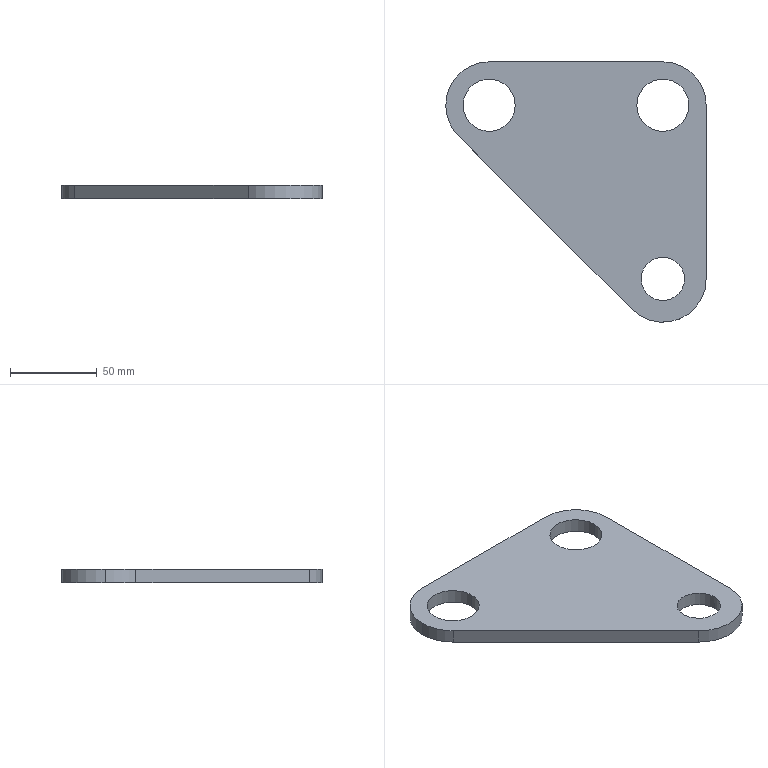Part | STEP file | 1 solid | 15 faces | box 150 x 150 x 8 mm | volume 108756 mm3 | cylinder 10 | plane 5 | commonest cylinder face diameters 30 x4 50 x4 25 x2
STEP:
#1=CARTESIAN_POINT('',(0.,0.,0.));
#2=DIRECTION('',(0.,0.,1.));
#3=DIRECTION('',(1.,0.,0.));
#4=AXIS2_PLACEMENT_3D('',#1,#2,#3);
#5=CARTESIAN_POINT('',(12.5,-100.,-4.));
#6=VERTEX_POINT('',#5);
#7=CARTESIAN_POINT('',(-12.5,-100.,-4.));
#8=VERTEX_POINT('',#7);
#9=CARTESIAN_POINT('',(0.,-100.,-4.));
#10=DIRECTION('',(0.,0.,1.));
#11=DIRECTION('',(1.,0.,0.));
#12=AXIS2_PLACEMENT_3D('',#9,#10,#11);
#13=CIRCLE('',#12,12.5);
#14=CARTESIAN_POINT('',(0.,-100.,4.));
#15=DIRECTION('',(0.,0.,-1.));
#16=DIRECTION('',(-1.,0.,0.));
#17=AXIS2_PLACEMENT_3D('',#14,#15,#16);
#18=CYLINDRICAL_SURFACE('',#17,12.5);
#19=CARTESIAN_POINT('',(3.142,8.));
#20=DIRECTION('',(-1.,0.));
#21=VECTOR('',#20,1.);
#22=LINE('',#19,#21);
#23=(GEOMETRIC_REPRESENTATION_CONTEXT(2)PARAMETRIC_REPRESENTATION_CONTEXT()REPRESENTATION_CONTEXT('',''));
#24=DEFINITIONAL_REPRESENTATION('',(#22),#23);
#25=PCURVE('',#18,#24);
#26=CARTESIAN_POINT('',(0.,-100.,-4.));
#27=DIRECTION('',(0.,0.,1.));
#28=DIRECTION('',(1.,0.,0.));
#29=AXIS2_PLACEMENT_3D('',#26,#27,#28);
#30=PLANE('',#29);
#31=CARTESIAN_POINT('',(0.,0.));
#32=DIRECTION('',(1.,0.));
#33=AXIS2_PLACEMENT_2D('',#31,#32);
#34=CIRCLE('',#33,12.5);
#35=(GEOMETRIC_REPRESENTATION_CONTEXT(2)PARAMETRIC_REPRESENTATION_CONTEXT()REPRESENTATION_CONTEXT('',''));
#36=DEFINITIONAL_REPRESENTATION('',(#34),#35);
#37=PCURVE('',#30,#36);
#38=SURFACE_CURVE('',#13,(#25,#37),.PCURVE_S1.);
#39=EDGE_CURVE('',#6,#8,#38,.T.);
#40=ORIENTED_EDGE('',*,*,#39,.T.);
#41=CARTESIAN_POINT('',(-12.5,-100.,4.));
#42=VERTEX_POINT('',#41);
#43=CARTESIAN_POINT('',(-12.5,-100.,4.));
#44=DIRECTION('',(0.,0.,-1.));
#45=VECTOR('',#44,1.);
#46=LINE('',#43,#45);
#47=CARTESIAN_POINT('',(0.,0.));
#48=DIRECTION('',(0.,1.));
#49=VECTOR('',#48,1.);
#50=LINE('',#47,#49);
#51=(GEOMETRIC_REPRESENTATION_CONTEXT(2)PARAMETRIC_REPRESENTATION_CONTEXT()REPRESENTATION_CONTEXT('',''));
#52=DEFINITIONAL_REPRESENTATION('',(#50),#51);
#53=PCURVE('',#18,#52);
#54=CARTESIAN_POINT('',(0.,-100.,4.));
#55=DIRECTION('',(0.,0.,-1.));
#56=DIRECTION('',(-1.,0.,0.));
#57=AXIS2_PLACEMENT_3D('',#54,#55,#56);
#58=CYLINDRICAL_SURFACE('',#57,12.5);
#59=CARTESIAN_POINT('',(6.283,0.));
#60=DIRECTION('',(0.,1.));
#61=VECTOR('',#60,1.);
#62=LINE('',#59,#61);
#63=(GEOMETRIC_REPRESENTATION_CONTEXT(2)PARAMETRIC_REPRESENTATION_CONTEXT()REPRESENTATION_CONTEXT('',''));
#64=DEFINITIONAL_REPRESENTATION('',(#62),#63);
#65=PCURVE('',#58,#64);
#66=SURFACE_CURVE('',#46,(#53,#65),.PCURVE_S1.);
#67=EDGE_CURVE('',#42,#8,#66,.T.);
#68=ORIENTED_EDGE('',*,*,#67,.F.);
#69=CARTESIAN_POINT('',(12.5,-100.,4.));
#70=VERTEX_POINT('',#69);
#71=CARTESIAN_POINT('',(0.,-100.,4.));
#72=DIRECTION('',(0.,0.,1.));
#73=DIRECTION('',(1.,0.,0.));
#74=AXIS2_PLACEMENT_3D('',#71,#72,#73);
#75=CIRCLE('',#74,12.5);
#76=CARTESIAN_POINT('',(3.142,0.));
#77=DIRECTION('',(-1.,0.));
#78=VECTOR('',#77,1.);
#79=LINE('',#76,#78);
#80=(GEOMETRIC_REPRESENTATION_CONTEXT(2)PARAMETRIC_REPRESENTATION_CONTEXT()REPRESENTATION_CONTEXT('',''));
#81=DEFINITIONAL_REPRESENTATION('',(#79),#80);
#82=PCURVE('',#18,#81);
#83=CARTESIAN_POINT('',(0.,-100.,4.));
#84=DIRECTION('',(0.,0.,1.));
#85=DIRECTION('',(1.,0.,0.));
#86=AXIS2_PLACEMENT_3D('',#83,#84,#85);
#87=PLANE('',#86);
#88=CARTESIAN_POINT('',(0.,0.));
#89=DIRECTION('',(1.,0.));
#90=AXIS2_PLACEMENT_2D('',#88,#89);
#91=CIRCLE('',#90,12.5);
#92=(GEOMETRIC_REPRESENTATION_CONTEXT(2)PARAMETRIC_REPRESENTATION_CONTEXT()REPRESENTATION_CONTEXT('',''));
#93=DEFINITIONAL_REPRESENTATION('',(#91),#92);
#94=PCURVE('',#87,#93);
#95=SURFACE_CURVE('',#75,(#82,#94),.PCURVE_S1.);
#96=EDGE_CURVE('',#70,#42,#95,.T.);
#97=ORIENTED_EDGE('',*,*,#96,.F.);
#98=CARTESIAN_POINT('',(12.5,-100.,4.));
#99=DIRECTION('',(0.,0.,-1.));
#100=VECTOR('',#99,1.);
#101=LINE('',#98,#100);
#102=CARTESIAN_POINT('',(3.142,0.));
#103=DIRECTION('',(0.,1.));
#104=VECTOR('',#103,1.);
#105=LINE('',#102,#104);
#106=(GEOMETRIC_REPRESENTATION_CONTEXT(2)PARAMETRIC_REPRESENTATION_CONTEXT()REPRESENTATION_CONTEXT('',''));
#107=DEFINITIONAL_REPRESENTATION('',(#105),#106);
#108=PCURVE('',#18,#107);
#109=CARTESIAN_POINT('',(3.142,0.));
#110=DIRECTION('',(0.,1.));
#111=VECTOR('',#110,1.);
#112=LINE('',#109,#111);
#113=(GEOMETRIC_REPRESENTATION_CONTEXT(2)PARAMETRIC_REPRESENTATION_CONTEXT()REPRESENTATION_CONTEXT('',''));
#114=DEFINITIONAL_REPRESENTATION('',(#112),#113);
#115=PCURVE('',#58,#114);
#116=SURFACE_CURVE('',#101,(#108,#115),.PCURVE_S1.);
#117=EDGE_CURVE('',#70,#6,#116,.T.);
#118=ORIENTED_EDGE('',*,*,#117,.T.);
#119=EDGE_LOOP('',(#40,#68,#97,#118));
#120=FACE_BOUND('',#119,.F.);
#121=ADVANCED_FACE('',(#120),#18,.F.);
#122=CARTESIAN_POINT('',(-85.,0.,-4.));
#123=VERTEX_POINT('',#122);
#124=CARTESIAN_POINT('',(-115.,0.,-4.));
#125=VERTEX_POINT('',#124);
#126=CARTESIAN_POINT('',(-100.,0.,-4.));
#127=DIRECTION('',(0.,0.,1.));
#128=DIRECTION('',(1.,0.,0.));
#129=AXIS2_PLACEMENT_3D('',#126,#127,#128);
#130=CIRCLE('',#129,15.);
#131=CARTESIAN_POINT('',(-100.,0.,4.));
#132=DIRECTION('',(0.,0.,-1.));
#133=DIRECTION('',(-1.,0.,0.));
#134=AXIS2_PLACEMENT_3D('',#131,#132,#133);
#135=CYLINDRICAL_SURFACE('',#134,15.);
#136=CARTESIAN_POINT('',(3.142,8.));
#137=DIRECTION('',(-1.,0.));
#138=VECTOR('',#137,1.);
#139=LINE('',#136,#138);
#140=(GEOMETRIC_REPRESENTATION_CONTEXT(2)PARAMETRIC_REPRESENTATION_CONTEXT()REPRESENTATION_CONTEXT('',''));
#141=DEFINITIONAL_REPRESENTATION('',(#139),#140);
#142=PCURVE('',#135,#141);
#143=CARTESIAN_POINT('',(-100.,100.));
#144=DIRECTION('',(1.,0.));
#145=AXIS2_PLACEMENT_2D('',#143,#144);
#146=CIRCLE('',#145,15.);
#147=(GEOMETRIC_REPRESENTATION_CONTEXT(2)PARAMETRIC_REPRESENTATION_CONTEXT()REPRESENTATION_CONTEXT('',''));
#148=DEFINITIONAL_REPRESENTATION('',(#146),#147);
#149=PCURVE('',#30,#148);
#150=SURFACE_CURVE('',#130,(#142,#149),.PCURVE_S1.);
#151=EDGE_CURVE('',#123,#125,#150,.T.);
#152=ORIENTED_EDGE('',*,*,#151,.T.);
#153=CARTESIAN_POINT('',(-115.,0.,4.));
#154=VERTEX_POINT('',#153);
#155=CARTESIAN_POINT('',(-115.,0.,4.));
#156=DIRECTION('',(0.,0.,-1.));
#157=VECTOR('',#156,1.);
#158=LINE('',#155,#157);
#159=CARTESIAN_POINT('',(0.,0.));
#160=DIRECTION('',(0.,1.));
#161=VECTOR('',#160,1.);
#162=LINE('',#159,#161);
#163=(GEOMETRIC_REPRESENTATION_CONTEXT(2)PARAMETRIC_REPRESENTATION_CONTEXT()REPRESENTATION_CONTEXT('',''));
#164=DEFINITIONAL_REPRESENTATION('',(#162),#163);
#165=PCURVE('',#135,#164);
#166=CARTESIAN_POINT('',(-100.,0.,4.));
#167=DIRECTION('',(0.,0.,-1.));
#168=DIRECTION('',(-1.,0.,0.));
#169=AXIS2_PLACEMENT_3D('',#166,#167,#168);
#170=CYLINDRICAL_SURFACE('',#169,15.);
#171=CARTESIAN_POINT('',(6.283,0.));
#172=DIRECTION('',(0.,1.));
#173=VECTOR('',#172,1.);
#174=LINE('',#171,#173);
#175=(GEOMETRIC_REPRESENTATION_CONTEXT(2)PARAMETRIC_REPRESENTATION_CONTEXT()REPRESENTATION_CONTEXT('',''));
#176=DEFINITIONAL_REPRESENTATION('',(#174),#175);
#177=PCURVE('',#170,#176);
#178=SURFACE_CURVE('',#158,(#165,#177),.PCURVE_S1.);
#179=EDGE_CURVE('',#154,#125,#178,.T.);
#180=ORIENTED_EDGE('',*,*,#179,.F.);
#181=CARTESIAN_POINT('',(-85.,0.,4.));
#182=VERTEX_POINT('',#181);
#183=CARTESIAN_POINT('',(-100.,0.,4.));
#184=DIRECTION('',(0.,0.,1.));
#185=DIRECTION('',(1.,0.,0.));
#186=AXIS2_PLACEMENT_3D('',#183,#184,#185);
#187=CIRCLE('',#186,15.);
#188=CARTESIAN_POINT('',(3.142,0.));
#189=DIRECTION('',(-1.,0.));
#190=VECTOR('',#189,1.);
#191=LINE('',#188,#190);
#192=(GEOMETRIC_REPRESENTATION_CONTEXT(2)PARAMETRIC_REPRESENTATION_CONTEXT()REPRESENTATION_CONTEXT('',''));
#193=DEFINITIONAL_REPRESENTATION('',(#191),#192);
#194=PCURVE('',#135,#193);
#195=CARTESIAN_POINT('',(-100.,100.));
#196=DIRECTION('',(1.,0.));
#197=AXIS2_PLACEMENT_2D('',#195,#196);
#198=CIRCLE('',#197,15.);
#199=(GEOMETRIC_REPRESENTATION_CONTEXT(2)PARAMETRIC_REPRESENTATION_CONTEXT()REPRESENTATION_CONTEXT('',''));
#200=DEFINITIONAL_REPRESENTATION('',(#198),#199);
#201=PCURVE('',#87,#200);
#202=SURFACE_CURVE('',#187,(#194,#201),.PCURVE_S1.);
#203=EDGE_CURVE('',#182,#154,#202,.T.);
#204=ORIENTED_EDGE('',*,*,#203,.F.);
#205=CARTESIAN_POINT('',(-85.,0.,4.));
#206=DIRECTION('',(0.,0.,-1.));
#207=VECTOR('',#206,1.);
#208=LINE('',#205,#207);
#209=CARTESIAN_POINT('',(3.142,0.));
#210=DIRECTION('',(0.,1.));
#211=VECTOR('',#210,1.);
#212=LINE('',#209,#211);
#213=(GEOMETRIC_REPRESENTATION_CONTEXT(2)PARAMETRIC_REPRESENTATION_CONTEXT()REPRESENTATION_CONTEXT('',''));
#214=DEFINITIONAL_REPRESENTATION('',(#212),#213);
#215=PCURVE('',#135,#214);
#216=CARTESIAN_POINT('',(3.142,0.));
#217=DIRECTION('',(0.,1.));
#218=VECTOR('',#217,1.);
#219=LINE('',#216,#218);
#220=(GEOMETRIC_REPRESENTATION_CONTEXT(2)PARAMETRIC_REPRESENTATION_CONTEXT()REPRESENTATION_CONTEXT('',''));
#221=DEFINITIONAL_REPRESENTATION('',(#219),#220);
#222=PCURVE('',#170,#221);
#223=SURFACE_CURVE('',#208,(#215,#222),.PCURVE_S1.);
#224=EDGE_CURVE('',#182,#123,#223,.T.);
#225=ORIENTED_EDGE('',*,*,#224,.T.);
#226=EDGE_LOOP('',(#152,#180,#204,#225));
#227=FACE_BOUND('',#226,.F.);
#228=ADVANCED_FACE('',(#227),#135,.F.);
#229=CARTESIAN_POINT('',(15.,0.,-4.));
#230=VERTEX_POINT('',#229);
#231=CARTESIAN_POINT('',(-15.,0.,-4.));
#232=VERTEX_POINT('',#231);
#233=CARTESIAN_POINT('',(0.,0.,-4.));
#234=DIRECTION('',(0.,0.,1.));
#235=DIRECTION('',(1.,0.,0.));
#236=AXIS2_PLACEMENT_3D('',#233,#234,#235);
#237=CIRCLE('',#236,15.);
#238=CARTESIAN_POINT('',(0.,0.,4.));
#239=DIRECTION('',(0.,0.,-1.));
#240=DIRECTION('',(-1.,0.,0.));
#241=AXIS2_PLACEMENT_3D('',#238,#239,#240);
#242=CYLINDRICAL_SURFACE('',#241,15.);
#243=CARTESIAN_POINT('',(3.142,8.));
#244=DIRECTION('',(-1.,0.));
#245=VECTOR('',#244,1.);
#246=LINE('',#243,#245);
#247=(GEOMETRIC_REPRESENTATION_CONTEXT(2)PARAMETRIC_REPRESENTATION_CONTEXT()REPRESENTATION_CONTEXT('',''));
#248=DEFINITIONAL_REPRESENTATION('',(#246),#247);
#249=PCURVE('',#242,#248);
#250=CARTESIAN_POINT('',(0.,100.));
#251=DIRECTION('',(1.,0.));
#252=AXIS2_PLACEMENT_2D('',#250,#251);
#253=CIRCLE('',#252,15.);
#254=(GEOMETRIC_REPRESENTATION_CONTEXT(2)PARAMETRIC_REPRESENTATION_CONTEXT()REPRESENTATION_CONTEXT('',''));
#255=DEFINITIONAL_REPRESENTATION('',(#253),#254);
#256=PCURVE('',#30,#255);
#257=SURFACE_CURVE('',#237,(#249,#256),.PCURVE_S1.);
#258=EDGE_CURVE('',#230,#232,#257,.T.);
#259=ORIENTED_EDGE('',*,*,#258,.T.);
#260=CARTESIAN_POINT('',(-15.,0.,4.));
#261=VERTEX_POINT('',#260);
#262=CARTESIAN_POINT('',(-15.,0.,4.));
#263=DIRECTION('',(0.,0.,-1.));
#264=VECTOR('',#263,1.);
#265=LINE('',#262,#264);
#266=CARTESIAN_POINT('',(0.,0.));
#267=DIRECTION('',(0.,1.));
#268=VECTOR('',#267,1.);
#269=LINE('',#266,#268);
#270=(GEOMETRIC_REPRESENTATION_CONTEXT(2)PARAMETRIC_REPRESENTATION_CONTEXT()REPRESENTATION_CONTEXT('',''));
#271=DEFINITIONAL_REPRESENTATION('',(#269),#270);
#272=PCURVE('',#242,#271);
#273=CARTESIAN_POINT('',(0.,0.,4.));
#274=DIRECTION('',(0.,0.,-1.));
#275=DIRECTION('',(-1.,0.,0.));
#276=AXIS2_PLACEMENT_3D('',#273,#274,#275);
#277=CYLINDRICAL_SURFACE('',#276,15.);
#278=CARTESIAN_POINT('',(6.283,0.));
#279=DIRECTION('',(0.,1.));
#280=VECTOR('',#279,1.);
#281=LINE('',#278,#280);
#282=(GEOMETRIC_REPRESENTATION_CONTEXT(2)PARAMETRIC_REPRESENTATION_CONTEXT()REPRESENTATION_CONTEXT('',''));
#283=DEFINITIONAL_REPRESENTATION('',(#281),#282);
#284=PCURVE('',#277,#283);
#285=SURFACE_CURVE('',#265,(#272,#284),.PCURVE_S1.);
#286=EDGE_CURVE('',#261,#232,#285,.T.);
#287=ORIENTED_EDGE('',*,*,#286,.F.);
#288=CARTESIAN_POINT('',(15.,0.,4.));
#289=VERTEX_POINT('',#288);
#290=CARTESIAN_POINT('',(0.,0.,4.));
#291=DIRECTION('',(0.,0.,1.));
#292=DIRECTION('',(1.,0.,0.));
#293=AXIS2_PLACEMENT_3D('',#290,#291,#292);
#294=CIRCLE('',#293,15.);
#295=CARTESIAN_POINT('',(3.142,0.));
#296=DIRECTION('',(-1.,0.));
#297=VECTOR('',#296,1.);
#298=LINE('',#295,#297);
#299=(GEOMETRIC_REPRESENTATION_CONTEXT(2)PARAMETRIC_REPRESENTATION_CONTEXT()REPRESENTATION_CONTEXT('',''));
#300=DEFINITIONAL_REPRESENTATION('',(#298),#299);
#301=PCURVE('',#242,#300);
#302=CARTESIAN_POINT('',(0.,100.));
#303=DIRECTION('',(1.,0.));
#304=AXIS2_PLACEMENT_2D('',#302,#303);
#305=CIRCLE('',#304,15.);
#306=(GEOMETRIC_REPRESENTATION_CONTEXT(2)PARAMETRIC_REPRESENTATION_CONTEXT()REPRESENTATION_CONTEXT('',''));
#307=DEFINITIONAL_REPRESENTATION('',(#305),#306);
#308=PCURVE('',#87,#307);
#309=SURFACE_CURVE('',#294,(#301,#308),.PCURVE_S1.);
#310=EDGE_CURVE('',#289,#261,#309,.T.);
#311=ORIENTED_EDGE('',*,*,#310,.F.);
#312=CARTESIAN_POINT('',(15.,0.,4.));
#313=DIRECTION('',(0.,0.,-1.));
#314=VECTOR('',#313,1.);
#315=LINE('',#312,#314);
#316=CARTESIAN_POINT('',(3.142,0.));
#317=DIRECTION('',(0.,1.));
#318=VECTOR('',#317,1.);
#319=LINE('',#316,#318);
#320=(GEOMETRIC_REPRESENTATION_CONTEXT(2)PARAMETRIC_REPRESENTATION_CONTEXT()REPRESENTATION_CONTEXT('',''));
#321=DEFINITIONAL_REPRESENTATION('',(#319),#320);
#322=PCURVE('',#242,#321);
#323=CARTESIAN_POINT('',(3.142,0.));
#324=DIRECTION('',(0.,1.));
#325=VECTOR('',#324,1.);
#326=LINE('',#323,#325);
#327=(GEOMETRIC_REPRESENTATION_CONTEXT(2)PARAMETRIC_REPRESENTATION_CONTEXT()REPRESENTATION_CONTEXT('',''));
#328=DEFINITIONAL_REPRESENTATION('',(#326),#327);
#329=PCURVE('',#277,#328);
#330=SURFACE_CURVE('',#315,(#322,#329),.PCURVE_S1.);
#331=EDGE_CURVE('',#289,#230,#330,.T.);
#332=ORIENTED_EDGE('',*,*,#331,.T.);
#333=EDGE_LOOP('',(#259,#287,#311,#332));
#334=FACE_BOUND('',#333,.F.);
#335=ADVANCED_FACE('',(#334),#242,.F.);
#336=CARTESIAN_POINT('',(-117.678,-17.678,-4.));
#337=VERTEX_POINT('',#336);
#338=CARTESIAN_POINT('',(-17.678,-117.678,-4.));
#339=VERTEX_POINT('',#338);
#340=CARTESIAN_POINT('',(-117.678,-17.678,-4.));
#341=DIRECTION('',(0.7071,-0.7071,0.));
#342=VECTOR('',#341,1.);
#343=LINE('',#340,#342);
#344=CARTESIAN_POINT('',(-117.678,-17.678,4.));
#345=DIRECTION('',(0.7071,0.7071,0.));
#346=DIRECTION('',(0.,0.,-1.));
#347=AXIS2_PLACEMENT_3D('',#344,#345,#346);
#348=PLANE('',#347);
#349=CARTESIAN_POINT('',(8.,0.));
#350=DIRECTION('',(0.,-1.));
#351=VECTOR('',#350,1.);
#352=LINE('',#349,#351);
#353=(GEOMETRIC_REPRESENTATION_CONTEXT(2)PARAMETRIC_REPRESENTATION_CONTEXT()REPRESENTATION_CONTEXT('',''));
#354=DEFINITIONAL_REPRESENTATION('',(#352),#353);
#355=PCURVE('',#348,#354);
#356=CARTESIAN_POINT('',(-117.678,82.322));
#357=DIRECTION('',(0.7071,-0.7071));
#358=VECTOR('',#357,1.);
#359=LINE('',#356,#358);
#360=(GEOMETRIC_REPRESENTATION_CONTEXT(2)PARAMETRIC_REPRESENTATION_CONTEXT()REPRESENTATION_CONTEXT('',''));
#361=DEFINITIONAL_REPRESENTATION('',(#359),#360);
#362=PCURVE('',#30,#361);
#363=SURFACE_CURVE('',#343,(#355,#362),.PCURVE_S1.);
#364=EDGE_CURVE('',#337,#339,#363,.T.);
#365=ORIENTED_EDGE('',*,*,#364,.T.);
#366=CARTESIAN_POINT('',(-17.678,-117.678,4.));
#367=VERTEX_POINT('',#366);
#368=CARTESIAN_POINT('',(-17.678,-117.678,4.));
#369=DIRECTION('',(0.,0.,-1.));
#370=VECTOR('',#369,1.);
#371=LINE('',#368,#370);
#372=CARTESIAN_POINT('',(0.,-141.421));
#373=DIRECTION('',(1.,0.));
#374=VECTOR('',#373,1.);
#375=LINE('',#372,#374);
#376=(GEOMETRIC_REPRESENTATION_CONTEXT(2)PARAMETRIC_REPRESENTATION_CONTEXT()REPRESENTATION_CONTEXT('',''));
#377=DEFINITIONAL_REPRESENTATION('',(#375),#376);
#378=PCURVE('',#348,#377);
#379=CARTESIAN_POINT('',(0.,-100.,4.));
#380=DIRECTION('',(0.,0.,-1.));
#381=DIRECTION('',(-1.,0.,0.));
#382=AXIS2_PLACEMENT_3D('',#379,#380,#381);
#383=CYLINDRICAL_SURFACE('',#382,25.);
#384=CARTESIAN_POINT('',(5.498,0.));
#385=DIRECTION('',(0.,1.));
#386=VECTOR('',#385,1.);
#387=LINE('',#384,#386);
#388=(GEOMETRIC_REPRESENTATION_CONTEXT(2)PARAMETRIC_REPRESENTATION_CONTEXT()REPRESENTATION_CONTEXT('',''));
#389=DEFINITIONAL_REPRESENTATION('',(#387),#388);
#390=PCURVE('',#383,#389);
#391=SURFACE_CURVE('',#371,(#378,#390),.PCURVE_S1.);
#392=EDGE_CURVE('',#367,#339,#391,.T.);
#393=ORIENTED_EDGE('',*,*,#392,.F.);
#394=CARTESIAN_POINT('',(-117.678,-17.678,4.));
#395=VERTEX_POINT('',#394);
#396=CARTESIAN_POINT('',(-117.678,-17.678,4.));
#397=DIRECTION('',(0.7071,-0.7071,0.));
#398=VECTOR('',#397,1.);
#399=LINE('',#396,#398);
#400=CARTESIAN_POINT('',(0.,0.));
#401=DIRECTION('',(0.,-1.));
#402=VECTOR('',#401,1.);
#403=LINE('',#400,#402);
#404=(GEOMETRIC_REPRESENTATION_CONTEXT(2)PARAMETRIC_REPRESENTATION_CONTEXT()REPRESENTATION_CONTEXT('',''));
#405=DEFINITIONAL_REPRESENTATION('',(#403),#404);
#406=PCURVE('',#348,#405);
#407=CARTESIAN_POINT('',(-117.678,82.322));
#408=DIRECTION('',(0.7071,-0.7071));
#409=VECTOR('',#408,1.);
#410=LINE('',#407,#409);
#411=(GEOMETRIC_REPRESENTATION_CONTEXT(2)PARAMETRIC_REPRESENTATION_CONTEXT()REPRESENTATION_CONTEXT('',''));
#412=DEFINITIONAL_REPRESENTATION('',(#410),#411);
#413=PCURVE('',#87,#412);
#414=SURFACE_CURVE('',#399,(#406,#413),.PCURVE_S1.);
#415=EDGE_CURVE('',#395,#367,#414,.T.);
#416=ORIENTED_EDGE('',*,*,#415,.F.);
#417=CARTESIAN_POINT('',(-117.678,-17.678,4.));
#418=DIRECTION('',(0.,0.,-1.));
#419=VECTOR('',#418,1.);
#420=LINE('',#417,#419);
#421=CARTESIAN_POINT('',(0.,0.));
#422=DIRECTION('',(1.,0.));
#423=VECTOR('',#422,1.);
#424=LINE('',#421,#423);
#425=(GEOMETRIC_REPRESENTATION_CONTEXT(2)PARAMETRIC_REPRESENTATION_CONTEXT()REPRESENTATION_CONTEXT('',''));
#426=DEFINITIONAL_REPRESENTATION('',(#424),#425);
#427=PCURVE('',#348,#426);
#428=CARTESIAN_POINT('',(-100.,0.,4.));
#429=DIRECTION('',(0.,0.,-1.));
#430=DIRECTION('',(-1.,0.,0.));
#431=AXIS2_PLACEMENT_3D('',#428,#429,#430);
#432=CYLINDRICAL_SURFACE('',#431,25.);
#433=CARTESIAN_POINT('',(5.498,0.));
#434=DIRECTION('',(0.,1.));
#435=VECTOR('',#434,1.);
#436=LINE('',#433,#435);
#437=(GEOMETRIC_REPRESENTATION_CONTEXT(2)PARAMETRIC_REPRESENTATION_CONTEXT()REPRESENTATION_CONTEXT('',''));
#438=DEFINITIONAL_REPRESENTATION('',(#436),#437);
#439=PCURVE('',#432,#438);
#440=SURFACE_CURVE('',#420,(#427,#439),.PCURVE_S1.);
#441=EDGE_CURVE('',#395,#337,#440,.T.);
#442=ORIENTED_EDGE('',*,*,#441,.T.);
#443=EDGE_LOOP('',(#365,#393,#416,#442));
#444=FACE_BOUND('',#443,.T.);
#445=ADVANCED_FACE('',(#444),#348,.F.);
#446=CARTESIAN_POINT('',(-125.,0.,4.));
#447=VERTEX_POINT('',#446);
#448=CARTESIAN_POINT('',(-125.,0.,-4.));
#449=VERTEX_POINT('',#448);
#450=CARTESIAN_POINT('',(-125.,0.,4.));
#451=DIRECTION('',(0.,0.,-1.));
#452=VECTOR('',#451,1.);
#453=LINE('',#450,#452);
#454=CARTESIAN_POINT('',(-100.,0.,4.));
#455=DIRECTION('',(0.,0.,-1.));
#456=DIRECTION('',(-1.,0.,0.));
#457=AXIS2_PLACEMENT_3D('',#454,#455,#456);
#458=CYLINDRICAL_SURFACE('',#457,25.);
#459=CARTESIAN_POINT('',(0.,0.));
#460=DIRECTION('',(0.,1.));
#461=VECTOR('',#460,1.);
#462=LINE('',#459,#461);
#463=(GEOMETRIC_REPRESENTATION_CONTEXT(2)PARAMETRIC_REPRESENTATION_CONTEXT()REPRESENTATION_CONTEXT('',''));
#464=DEFINITIONAL_REPRESENTATION('',(#462),#463);
#465=PCURVE('',#458,#464);
#466=CARTESIAN_POINT('',(6.283,0.));
#467=DIRECTION('',(0.,1.));
#468=VECTOR('',#467,1.);
#469=LINE('',#466,#468);
#470=(GEOMETRIC_REPRESENTATION_CONTEXT(2)PARAMETRIC_REPRESENTATION_CONTEXT()REPRESENTATION_CONTEXT('',''));
#471=DEFINITIONAL_REPRESENTATION('',(#469),#470);
#472=PCURVE('',#432,#471);
#473=SURFACE_CURVE('',#453,(#465,#472),.PCURVE_S1.);
#474=EDGE_CURVE('',#447,#449,#473,.T.);
#475=ORIENTED_EDGE('',*,*,#474,.F.);
#476=CARTESIAN_POINT('',(-100.,25.,4.));
#477=VERTEX_POINT('',#476);
#478=CARTESIAN_POINT('',(-100.,0.,4.));
#479=DIRECTION('',(0.,0.,1.));
#480=DIRECTION('',(1.,0.,0.));
#481=AXIS2_PLACEMENT_3D('',#478,#479,#480);
#482=CIRCLE('',#481,25.);
#483=CARTESIAN_POINT('',(3.142,0.));
#484=DIRECTION('',(-1.,0.));
#485=VECTOR('',#484,1.);
#486=LINE('',#483,#485);
#487=(GEOMETRIC_REPRESENTATION_CONTEXT(2)PARAMETRIC_REPRESENTATION_CONTEXT()REPRESENTATION_CONTEXT('',''));
#488=DEFINITIONAL_REPRESENTATION('',(#486),#487);
#489=PCURVE('',#458,#488);
#490=CARTESIAN_POINT('',(-100.,100.));
#491=DIRECTION('',(1.,0.));
#492=AXIS2_PLACEMENT_2D('',#490,#491);
#493=CIRCLE('',#492,25.);
#494=(GEOMETRIC_REPRESENTATION_CONTEXT(2)PARAMETRIC_REPRESENTATION_CONTEXT()REPRESENTATION_CONTEXT('',''));
#495=DEFINITIONAL_REPRESENTATION('',(#493),#494);
#496=PCURVE('',#87,#495);
#497=SURFACE_CURVE('',#482,(#489,#496),.PCURVE_S1.);
#498=EDGE_CURVE('',#477,#447,#497,.T.);
#499=ORIENTED_EDGE('',*,*,#498,.F.);
#500=CARTESIAN_POINT('',(-100.,25.,-4.));
#501=VERTEX_POINT('',#500);
#502=CARTESIAN_POINT('',(-100.,25.,4.));
#503=DIRECTION('',(0.,0.,-1.));
#504=VECTOR('',#503,1.);
#505=LINE('',#502,#504);
#506=CARTESIAN_POINT('',(1.571,0.));
#507=DIRECTION('',(0.,1.));
#508=VECTOR('',#507,1.);
#509=LINE('',#506,#508);
#510=(GEOMETRIC_REPRESENTATION_CONTEXT(2)PARAMETRIC_REPRESENTATION_CONTEXT()REPRESENTATION_CONTEXT('',''));
#511=DEFINITIONAL_REPRESENTATION('',(#509),#510);
#512=PCURVE('',#458,#511);
#513=CARTESIAN_POINT('',(-100.,25.,4.));
#514=DIRECTION('',(0.,-1.,0.));
#515=DIRECTION('',(0.,0.,-1.));
#516=AXIS2_PLACEMENT_3D('',#513,#514,#515);
#517=PLANE('',#516);
#518=CARTESIAN_POINT('',(0.,0.));
#519=DIRECTION('',(1.,0.));
#520=VECTOR('',#519,1.);
#521=LINE('',#518,#520);
#522=(GEOMETRIC_REPRESENTATION_CONTEXT(2)PARAMETRIC_REPRESENTATION_CONTEXT()REPRESENTATION_CONTEXT('',''));
#523=DEFINITIONAL_REPRESENTATION('',(#521),#522);
#524=PCURVE('',#517,#523);
#525=SURFACE_CURVE('',#505,(#512,#524),.PCURVE_S1.);
#526=EDGE_CURVE('',#477,#501,#525,.T.);
#527=ORIENTED_EDGE('',*,*,#526,.T.);
#528=CARTESIAN_POINT('',(-100.,0.,-4.));
#529=DIRECTION('',(0.,0.,1.));
#530=DIRECTION('',(1.,0.,0.));
#531=AXIS2_PLACEMENT_3D('',#528,#529,#530);
#532=CIRCLE('',#531,25.);
#533=CARTESIAN_POINT('',(3.142,8.));
#534=DIRECTION('',(-1.,0.));
#535=VECTOR('',#534,1.);
#536=LINE('',#533,#535);
#537=(GEOMETRIC_REPRESENTATION_CONTEXT(2)PARAMETRIC_REPRESENTATION_CONTEXT()REPRESENTATION_CONTEXT('',''));
#538=DEFINITIONAL_REPRESENTATION('',(#536),#537);
#539=PCURVE('',#458,#538);
#540=CARTESIAN_POINT('',(-100.,100.));
#541=DIRECTION('',(1.,0.));
#542=AXIS2_PLACEMENT_2D('',#540,#541);
#543=CIRCLE('',#542,25.);
#544=(GEOMETRIC_REPRESENTATION_CONTEXT(2)PARAMETRIC_REPRESENTATION_CONTEXT()REPRESENTATION_CONTEXT('',''));
#545=DEFINITIONAL_REPRESENTATION('',(#543),#544);
#546=PCURVE('',#30,#545);
#547=SURFACE_CURVE('',#532,(#539,#546),.PCURVE_S1.);
#548=EDGE_CURVE('',#501,#449,#547,.T.);
#549=ORIENTED_EDGE('',*,*,#548,.T.);
#550=EDGE_LOOP('',(#475,#499,#527,#549));
#551=FACE_BOUND('',#550,.T.);
#552=ADVANCED_FACE('',(#551),#458,.T.);
#553=CARTESIAN_POINT('',(0.,25.,-4.));
#554=VERTEX_POINT('',#553);
#555=CARTESIAN_POINT('',(-100.,25.,-4.));
#556=DIRECTION('',(-1.,0.,0.));
#557=VECTOR('',#556,1.);
#558=LINE('',#555,#557);
#559=CARTESIAN_POINT('',(8.,0.));
#560=DIRECTION('',(0.,-1.));
#561=VECTOR('',#560,1.);
#562=LINE('',#559,#561);
#563=(GEOMETRIC_REPRESENTATION_CONTEXT(2)PARAMETRIC_REPRESENTATION_CONTEXT()REPRESENTATION_CONTEXT('',''));
#564=DEFINITIONAL_REPRESENTATION('',(#562),#563);
#565=PCURVE('',#517,#564);
#566=CARTESIAN_POINT('',(-100.,125.));
#567=DIRECTION('',(-1.,0.));
#568=VECTOR('',#567,1.);
#569=LINE('',#566,#568);
#570=(GEOMETRIC_REPRESENTATION_CONTEXT(2)PARAMETRIC_REPRESENTATION_CONTEXT()REPRESENTATION_CONTEXT('',''));
#571=DEFINITIONAL_REPRESENTATION('',(#569),#570);
#572=PCURVE('',#30,#571);
#573=SURFACE_CURVE('',#558,(#565,#572),.PCURVE_S1.);
#574=EDGE_CURVE('',#554,#501,#573,.T.);
#575=ORIENTED_EDGE('',*,*,#574,.T.);
#576=ORIENTED_EDGE('',*,*,#526,.F.);
#577=CARTESIAN_POINT('',(0.,25.,4.));
#578=VERTEX_POINT('',#577);
#579=CARTESIAN_POINT('',(-100.,25.,4.));
#580=DIRECTION('',(-1.,0.,0.));
#581=VECTOR('',#580,1.);
#582=LINE('',#579,#581);
#583=CARTESIAN_POINT('',(0.,0.));
#584=DIRECTION('',(0.,-1.));
#585=VECTOR('',#584,1.);
#586=LINE('',#583,#585);
#587=(GEOMETRIC_REPRESENTATION_CONTEXT(2)PARAMETRIC_REPRESENTATION_CONTEXT()REPRESENTATION_CONTEXT('',''));
#588=DEFINITIONAL_REPRESENTATION('',(#586),#587);
#589=PCURVE('',#517,#588);
#590=CARTESIAN_POINT('',(-100.,125.));
#591=DIRECTION('',(-1.,0.));
#592=VECTOR('',#591,1.);
#593=LINE('',#590,#592);
#594=(GEOMETRIC_REPRESENTATION_CONTEXT(2)PARAMETRIC_REPRESENTATION_CONTEXT()REPRESENTATION_CONTEXT('',''));
#595=DEFINITIONAL_REPRESENTATION('',(#593),#594);
#596=PCURVE('',#87,#595);
#597=SURFACE_CURVE('',#582,(#589,#596),.PCURVE_S1.);
#598=EDGE_CURVE('',#578,#477,#597,.T.);
#599=ORIENTED_EDGE('',*,*,#598,.F.);
#600=CARTESIAN_POINT('',(0.,25.,4.));
#601=DIRECTION('',(0.,0.,-1.));
#602=VECTOR('',#601,1.);
#603=LINE('',#600,#602);
#604=CARTESIAN_POINT('',(0.,100.));
#605=DIRECTION('',(1.,0.));
#606=VECTOR('',#605,1.);
#607=LINE('',#604,#606);
#608=(GEOMETRIC_REPRESENTATION_CONTEXT(2)PARAMETRIC_REPRESENTATION_CONTEXT()REPRESENTATION_CONTEXT('',''));
#609=DEFINITIONAL_REPRESENTATION('',(#607),#608);
#610=PCURVE('',#517,#609);
#611=CARTESIAN_POINT('',(0.,0.,4.));
#612=DIRECTION('',(0.,0.,-1.));
#613=DIRECTION('',(-1.,0.,0.));
#614=AXIS2_PLACEMENT_3D('',#611,#612,#613);
#615=CYLINDRICAL_SURFACE('',#614,25.);
#616=CARTESIAN_POINT('',(1.571,0.));
#617=DIRECTION('',(0.,1.));
#618=VECTOR('',#617,1.);
#619=LINE('',#616,#618);
#620=(GEOMETRIC_REPRESENTATION_CONTEXT(2)PARAMETRIC_REPRESENTATION_CONTEXT()REPRESENTATION_CONTEXT('',''));
#621=DEFINITIONAL_REPRESENTATION('',(#619),#620);
#622=PCURVE('',#615,#621);
#623=SURFACE_CURVE('',#603,(#610,#622),.PCURVE_S1.);
#624=EDGE_CURVE('',#578,#554,#623,.T.);
#625=ORIENTED_EDGE('',*,*,#624,.T.);
#626=EDGE_LOOP('',(#575,#576,#599,#625));
#627=FACE_BOUND('',#626,.T.);
#628=ADVANCED_FACE('',(#627),#517,.F.);
#629=CARTESIAN_POINT('',(25.,0.,-4.));
#630=VERTEX_POINT('',#629);
#631=CARTESIAN_POINT('',(0.,0.,-4.));
#632=DIRECTION('',(0.,0.,1.));
#633=DIRECTION('',(1.,0.,0.));
#634=AXIS2_PLACEMENT_3D('',#631,#632,#633);
#635=CIRCLE('',#634,25.);
#636=CARTESIAN_POINT('',(3.142,8.));
#637=DIRECTION('',(-1.,0.));
#638=VECTOR('',#637,1.);
#639=LINE('',#636,#638);
#640=(GEOMETRIC_REPRESENTATION_CONTEXT(2)PARAMETRIC_REPRESENTATION_CONTEXT()REPRESENTATION_CONTEXT('',''));
#641=DEFINITIONAL_REPRESENTATION('',(#639),#640);
#642=PCURVE('',#615,#641);
#643=CARTESIAN_POINT('',(0.,100.));
#644=DIRECTION('',(1.,0.));
#645=AXIS2_PLACEMENT_2D('',#643,#644);
#646=CIRCLE('',#645,25.);
#647=(GEOMETRIC_REPRESENTATION_CONTEXT(2)PARAMETRIC_REPRESENTATION_CONTEXT()REPRESENTATION_CONTEXT('',''));
#648=DEFINITIONAL_REPRESENTATION('',(#646),#647);
#649=PCURVE('',#30,#648);
#650=SURFACE_CURVE('',#635,(#642,#649),.PCURVE_S1.);
#651=EDGE_CURVE('',#630,#554,#650,.T.);
#652=ORIENTED_EDGE('',*,*,#651,.T.);
#653=ORIENTED_EDGE('',*,*,#624,.F.);
#654=CARTESIAN_POINT('',(25.,0.,4.));
#655=VERTEX_POINT('',#654);
#656=CARTESIAN_POINT('',(0.,0.,4.));
#657=DIRECTION('',(0.,0.,1.));
#658=DIRECTION('',(1.,0.,0.));
#659=AXIS2_PLACEMENT_3D('',#656,#657,#658);
#660=CIRCLE('',#659,25.);
#661=CARTESIAN_POINT('',(3.142,0.));
#662=DIRECTION('',(-1.,0.));
#663=VECTOR('',#662,1.);
#664=LINE('',#661,#663);
#665=(GEOMETRIC_REPRESENTATION_CONTEXT(2)PARAMETRIC_REPRESENTATION_CONTEXT()REPRESENTATION_CONTEXT('',''));
#666=DEFINITIONAL_REPRESENTATION('',(#664),#665);
#667=PCURVE('',#615,#666);
#668=CARTESIAN_POINT('',(0.,100.));
#669=DIRECTION('',(1.,0.));
#670=AXIS2_PLACEMENT_2D('',#668,#669);
#671=CIRCLE('',#670,25.);
#672=(GEOMETRIC_REPRESENTATION_CONTEXT(2)PARAMETRIC_REPRESENTATION_CONTEXT()REPRESENTATION_CONTEXT('',''));
#673=DEFINITIONAL_REPRESENTATION('',(#671),#672);
#674=PCURVE('',#87,#673);
#675=SURFACE_CURVE('',#660,(#667,#674),.PCURVE_S1.);
#676=EDGE_CURVE('',#655,#578,#675,.T.);
#677=ORIENTED_EDGE('',*,*,#676,.F.);
#678=CARTESIAN_POINT('',(25.,0.,4.));
#679=DIRECTION('',(0.,0.,-1.));
#680=VECTOR('',#679,1.);
#681=LINE('',#678,#680);
#682=CARTESIAN_POINT('',(3.142,0.));
#683=DIRECTION('',(0.,1.));
#684=VECTOR('',#683,1.);
#685=LINE('',#682,#684);
#686=(GEOMETRIC_REPRESENTATION_CONTEXT(2)PARAMETRIC_REPRESENTATION_CONTEXT()REPRESENTATION_CONTEXT('',''));
#687=DEFINITIONAL_REPRESENTATION('',(#685),#686);
#688=PCURVE('',#615,#687);
#689=CARTESIAN_POINT('',(25.,0.,4.));
#690=DIRECTION('',(-1.,0.,0.));
#691=DIRECTION('',(0.,1.,0.));
#692=AXIS2_PLACEMENT_3D('',#689,#690,#691);
#693=PLANE('',#692);
#694=CARTESIAN_POINT('',(0.,0.));
#695=DIRECTION('',(0.,1.));
#696=VECTOR('',#695,1.);
#697=LINE('',#694,#696);
#698=(GEOMETRIC_REPRESENTATION_CONTEXT(2)PARAMETRIC_REPRESENTATION_CONTEXT()REPRESENTATION_CONTEXT('',''));
#699=DEFINITIONAL_REPRESENTATION('',(#697),#698);
#700=PCURVE('',#693,#699);
#701=SURFACE_CURVE('',#681,(#688,#700),.PCURVE_S1.);
#702=EDGE_CURVE('',#655,#630,#701,.T.);
#703=ORIENTED_EDGE('',*,*,#702,.T.);
#704=EDGE_LOOP('',(#652,#653,#677,#703));
#705=FACE_BOUND('',#704,.T.);
#706=ADVANCED_FACE('',(#705),#615,.T.);
#707=CARTESIAN_POINT('',(25.,-100.,-4.));
#708=VERTEX_POINT('',#707);
#709=CARTESIAN_POINT('',(25.,0.,-4.));
#710=DIRECTION('',(0.,1.,0.));
#711=VECTOR('',#710,1.);
#712=LINE('',#709,#711);
#713=CARTESIAN_POINT('',(0.,8.));
#714=DIRECTION('',(1.,0.));
#715=VECTOR('',#714,1.);
#716=LINE('',#713,#715);
#717=(GEOMETRIC_REPRESENTATION_CONTEXT(2)PARAMETRIC_REPRESENTATION_CONTEXT()REPRESENTATION_CONTEXT('',''));
#718=DEFINITIONAL_REPRESENTATION('',(#716),#717);
#719=PCURVE('',#693,#718);
#720=CARTESIAN_POINT('',(25.,100.));
#721=DIRECTION('',(0.,1.));
#722=VECTOR('',#721,1.);
#723=LINE('',#720,#722);
#724=(GEOMETRIC_REPRESENTATION_CONTEXT(2)PARAMETRIC_REPRESENTATION_CONTEXT()REPRESENTATION_CONTEXT('',''));
#725=DEFINITIONAL_REPRESENTATION('',(#723),#724);
#726=PCURVE('',#30,#725);
#727=SURFACE_CURVE('',#712,(#719,#726),.PCURVE_S1.);
#728=EDGE_CURVE('',#708,#630,#727,.T.);
#729=ORIENTED_EDGE('',*,*,#728,.T.);
#730=ORIENTED_EDGE('',*,*,#702,.F.);
#731=CARTESIAN_POINT('',(25.,-100.,4.));
#732=VERTEX_POINT('',#731);
#733=CARTESIAN_POINT('',(25.,0.,4.));
#734=DIRECTION('',(0.,1.,0.));
#735=VECTOR('',#734,1.);
#736=LINE('',#733,#735);
#737=CARTESIAN_POINT('',(0.,0.));
#738=DIRECTION('',(1.,0.));
#739=VECTOR('',#738,1.);
#740=LINE('',#737,#739);
#741=(GEOMETRIC_REPRESENTATION_CONTEXT(2)PARAMETRIC_REPRESENTATION_CONTEXT()REPRESENTATION_CONTEXT('',''));
#742=DEFINITIONAL_REPRESENTATION('',(#740),#741);
#743=PCURVE('',#693,#742);
#744=CARTESIAN_POINT('',(25.,100.));
#745=DIRECTION('',(0.,1.));
#746=VECTOR('',#745,1.);
#747=LINE('',#744,#746);
#748=(GEOMETRIC_REPRESENTATION_CONTEXT(2)PARAMETRIC_REPRESENTATION_CONTEXT()REPRESENTATION_CONTEXT('',''));
#749=DEFINITIONAL_REPRESENTATION('',(#747),#748);
#750=PCURVE('',#87,#749);
#751=SURFACE_CURVE('',#736,(#743,#750),.PCURVE_S1.);
#752=EDGE_CURVE('',#732,#655,#751,.T.);
#753=ORIENTED_EDGE('',*,*,#752,.F.);
#754=CARTESIAN_POINT('',(25.,-100.,4.));
#755=DIRECTION('',(0.,0.,-1.));
#756=VECTOR('',#755,1.);
#757=LINE('',#754,#756);
#758=CARTESIAN_POINT('',(-100.,0.));
#759=DIRECTION('',(0.,1.));
#760=VECTOR('',#759,1.);
#761=LINE('',#758,#760);
#762=(GEOMETRIC_REPRESENTATION_CONTEXT(2)PARAMETRIC_REPRESENTATION_CONTEXT()REPRESENTATION_CONTEXT('',''));
#763=DEFINITIONAL_REPRESENTATION('',(#761),#762);
#764=PCURVE('',#693,#763);
#765=CARTESIAN_POINT('',(3.142,0.));
#766=DIRECTION('',(0.,1.));
#767=VECTOR('',#766,1.);
#768=LINE('',#765,#767);
#769=(GEOMETRIC_REPRESENTATION_CONTEXT(2)PARAMETRIC_REPRESENTATION_CONTEXT()REPRESENTATION_CONTEXT('',''));
#770=DEFINITIONAL_REPRESENTATION('',(#768),#769);
#771=PCURVE('',#383,#770);
#772=SURFACE_CURVE('',#757,(#764,#771),.PCURVE_S1.);
#773=EDGE_CURVE('',#732,#708,#772,.T.);
#774=ORIENTED_EDGE('',*,*,#773,.T.);
#775=EDGE_LOOP('',(#729,#730,#753,#774));
#776=FACE_BOUND('',#775,.T.);
#777=ADVANCED_FACE('',(#776),#693,.F.);
#778=CARTESIAN_POINT('',(0.,-100.,-4.));
#779=DIRECTION('',(0.,0.,1.));
#780=DIRECTION('',(1.,0.,0.));
#781=AXIS2_PLACEMENT_3D('',#778,#779,#780);
#782=CIRCLE('',#781,25.);
#783=CARTESIAN_POINT('',(9.425,8.));
#784=DIRECTION('',(-1.,0.));
#785=VECTOR('',#784,1.);
#786=LINE('',#783,#785);
#787=(GEOMETRIC_REPRESENTATION_CONTEXT(2)PARAMETRIC_REPRESENTATION_CONTEXT()REPRESENTATION_CONTEXT('',''));
#788=DEFINITIONAL_REPRESENTATION('',(#786),#787);
#789=PCURVE('',#383,#788);
#790=CARTESIAN_POINT('',(0.,0.));
#791=DIRECTION('',(1.,0.));
#792=AXIS2_PLACEMENT_2D('',#790,#791);
#793=CIRCLE('',#792,25.);
#794=(GEOMETRIC_REPRESENTATION_CONTEXT(2)PARAMETRIC_REPRESENTATION_CONTEXT()REPRESENTATION_CONTEXT('',''));
#795=DEFINITIONAL_REPRESENTATION('',(#793),#794);
#796=PCURVE('',#30,#795);
#797=SURFACE_CURVE('',#782,(#789,#796),.PCURVE_S1.);
#798=EDGE_CURVE('',#339,#708,#797,.T.);
#799=ORIENTED_EDGE('',*,*,#798,.T.);
#800=ORIENTED_EDGE('',*,*,#773,.F.);
#801=CARTESIAN_POINT('',(0.,-100.,4.));
#802=DIRECTION('',(0.,0.,1.));
#803=DIRECTION('',(1.,0.,0.));
#804=AXIS2_PLACEMENT_3D('',#801,#802,#803);
#805=CIRCLE('',#804,25.);
#806=CARTESIAN_POINT('',(9.425,0.));
#807=DIRECTION('',(-1.,0.));
#808=VECTOR('',#807,1.);
#809=LINE('',#806,#808);
#810=(GEOMETRIC_REPRESENTATION_CONTEXT(2)PARAMETRIC_REPRESENTATION_CONTEXT()REPRESENTATION_CONTEXT('',''));
#811=DEFINITIONAL_REPRESENTATION('',(#809),#810);
#812=PCURVE('',#383,#811);
#813=CARTESIAN_POINT('',(0.,0.));
#814=DIRECTION('',(1.,0.));
#815=AXIS2_PLACEMENT_2D('',#813,#814);
#816=CIRCLE('',#815,25.);
#817=(GEOMETRIC_REPRESENTATION_CONTEXT(2)PARAMETRIC_REPRESENTATION_CONTEXT()REPRESENTATION_CONTEXT('',''));
#818=DEFINITIONAL_REPRESENTATION('',(#816),#817);
#819=PCURVE('',#87,#818);
#820=SURFACE_CURVE('',#805,(#812,#819),.PCURVE_S1.);
#821=EDGE_CURVE('',#367,#732,#820,.T.);
#822=ORIENTED_EDGE('',*,*,#821,.F.);
#823=ORIENTED_EDGE('',*,*,#392,.T.);
#824=EDGE_LOOP('',(#799,#800,#822,#823));
#825=FACE_BOUND('',#824,.T.);
#826=ADVANCED_FACE('',(#825),#383,.T.);
#827=CARTESIAN_POINT('',(0.,-100.,-4.));
#828=DIRECTION('',(0.,0.,1.));
#829=DIRECTION('',(1.,0.,0.));
#830=AXIS2_PLACEMENT_3D('',#827,#828,#829);
#831=CIRCLE('',#830,12.5);
#832=CARTESIAN_POINT('',(0.,0.));
#833=DIRECTION('',(1.,0.));
#834=AXIS2_PLACEMENT_2D('',#832,#833);
#835=CIRCLE('',#834,12.5);
#836=(GEOMETRIC_REPRESENTATION_CONTEXT(2)PARAMETRIC_REPRESENTATION_CONTEXT()REPRESENTATION_CONTEXT('',''));
#837=DEFINITIONAL_REPRESENTATION('',(#835),#836);
#838=PCURVE('',#30,#837);
#839=CARTESIAN_POINT('',(9.425,8.));
#840=DIRECTION('',(-1.,0.));
#841=VECTOR('',#840,1.);
#842=LINE('',#839,#841);
#843=(GEOMETRIC_REPRESENTATION_CONTEXT(2)PARAMETRIC_REPRESENTATION_CONTEXT()REPRESENTATION_CONTEXT('',''));
#844=DEFINITIONAL_REPRESENTATION('',(#842),#843);
#845=PCURVE('',#58,#844);
#846=SURFACE_CURVE('',#831,(#838,#845),.PCURVE_S1.);
#847=EDGE_CURVE('',#8,#6,#846,.T.);
#848=ORIENTED_EDGE('',*,*,#847,.T.);
#849=ORIENTED_EDGE('',*,*,#39,.T.);
#850=EDGE_LOOP('',(#848,#849));
#851=FACE_BOUND('',#850,.T.);
#852=CARTESIAN_POINT('',(0.,0.,-4.));
#853=DIRECTION('',(0.,0.,1.));
#854=DIRECTION('',(1.,0.,0.));
#855=AXIS2_PLACEMENT_3D('',#852,#853,#854);
#856=CIRCLE('',#855,15.);
#857=CARTESIAN_POINT('',(0.,100.));
#858=DIRECTION('',(1.,0.));
#859=AXIS2_PLACEMENT_2D('',#857,#858);
#860=CIRCLE('',#859,15.);
#861=(GEOMETRIC_REPRESENTATION_CONTEXT(2)PARAMETRIC_REPRESENTATION_CONTEXT()REPRESENTATION_CONTEXT('',''));
#862=DEFINITIONAL_REPRESENTATION('',(#860),#861);
#863=PCURVE('',#30,#862);
#864=CARTESIAN_POINT('',(9.425,8.));
#865=DIRECTION('',(-1.,0.));
#866=VECTOR('',#865,1.);
#867=LINE('',#864,#866);
#868=(GEOMETRIC_REPRESENTATION_CONTEXT(2)PARAMETRIC_REPRESENTATION_CONTEXT()REPRESENTATION_CONTEXT('',''));
#869=DEFINITIONAL_REPRESENTATION('',(#867),#868);
#870=PCURVE('',#277,#869);
#871=SURFACE_CURVE('',#856,(#863,#870),.PCURVE_S1.);
#872=EDGE_CURVE('',#232,#230,#871,.T.);
#873=ORIENTED_EDGE('',*,*,#872,.T.);
#874=ORIENTED_EDGE('',*,*,#258,.T.);
#875=EDGE_LOOP('',(#873,#874));
#876=FACE_BOUND('',#875,.T.);
#877=CARTESIAN_POINT('',(-100.,0.,-4.));
#878=DIRECTION('',(0.,0.,1.));
#879=DIRECTION('',(1.,0.,0.));
#880=AXIS2_PLACEMENT_3D('',#877,#878,#879);
#881=CIRCLE('',#880,15.);
#882=CARTESIAN_POINT('',(-100.,100.));
#883=DIRECTION('',(1.,0.));
#884=AXIS2_PLACEMENT_2D('',#882,#883);
#885=CIRCLE('',#884,15.);
#886=(GEOMETRIC_REPRESENTATION_CONTEXT(2)PARAMETRIC_REPRESENTATION_CONTEXT()REPRESENTATION_CONTEXT('',''));
#887=DEFINITIONAL_REPRESENTATION('',(#885),#886);
#888=PCURVE('',#30,#887);
#889=CARTESIAN_POINT('',(9.425,8.));
#890=DIRECTION('',(-1.,0.));
#891=VECTOR('',#890,1.);
#892=LINE('',#889,#891);
#893=(GEOMETRIC_REPRESENTATION_CONTEXT(2)PARAMETRIC_REPRESENTATION_CONTEXT()REPRESENTATION_CONTEXT('',''));
#894=DEFINITIONAL_REPRESENTATION('',(#892),#893);
#895=PCURVE('',#170,#894);
#896=SURFACE_CURVE('',#881,(#888,#895),.PCURVE_S1.);
#897=EDGE_CURVE('',#125,#123,#896,.T.);
#898=ORIENTED_EDGE('',*,*,#897,.T.);
#899=ORIENTED_EDGE('',*,*,#151,.T.);
#900=EDGE_LOOP('',(#898,#899));
#901=FACE_BOUND('',#900,.T.);
#902=ORIENTED_EDGE('',*,*,#798,.F.);
#903=ORIENTED_EDGE('',*,*,#364,.F.);
#904=CARTESIAN_POINT('',(-100.,0.,-4.));
#905=DIRECTION('',(0.,0.,1.));
#906=DIRECTION('',(1.,0.,0.));
#907=AXIS2_PLACEMENT_3D('',#904,#905,#906);
#908=CIRCLE('',#907,25.);
#909=CARTESIAN_POINT('',(-100.,100.));
#910=DIRECTION('',(1.,0.));
#911=AXIS2_PLACEMENT_2D('',#909,#910);
#912=CIRCLE('',#911,25.);
#913=(GEOMETRIC_REPRESENTATION_CONTEXT(2)PARAMETRIC_REPRESENTATION_CONTEXT()REPRESENTATION_CONTEXT('',''));
#914=DEFINITIONAL_REPRESENTATION('',(#912),#913);
#915=PCURVE('',#30,#914);
#916=CARTESIAN_POINT('',(9.425,8.));
#917=DIRECTION('',(-1.,0.));
#918=VECTOR('',#917,1.);
#919=LINE('',#916,#918);
#920=(GEOMETRIC_REPRESENTATION_CONTEXT(2)PARAMETRIC_REPRESENTATION_CONTEXT()REPRESENTATION_CONTEXT('',''));
#921=DEFINITIONAL_REPRESENTATION('',(#919),#920);
#922=PCURVE('',#432,#921);
#923=SURFACE_CURVE('',#908,(#915,#922),.PCURVE_S1.);
#924=EDGE_CURVE('',#449,#337,#923,.T.);
#925=ORIENTED_EDGE('',*,*,#924,.F.);
#926=ORIENTED_EDGE('',*,*,#548,.F.);
#927=ORIENTED_EDGE('',*,*,#574,.F.);
#928=ORIENTED_EDGE('',*,*,#651,.F.);
#929=ORIENTED_EDGE('',*,*,#728,.F.);
#930=EDGE_LOOP('',(#902,#903,#925,#926,#927,#928,#929));
#931=FACE_BOUND('',#930,.T.);
#932=ADVANCED_FACE('',(#851,#876,#901,#931),#30,.F.);
#933=CARTESIAN_POINT('',(0.,-100.,4.));
#934=DIRECTION('',(0.,0.,1.));
#935=DIRECTION('',(1.,0.,0.));
#936=AXIS2_PLACEMENT_3D('',#933,#934,#935);
#937=CIRCLE('',#936,12.5);
#938=CARTESIAN_POINT('',(0.,0.));
#939=DIRECTION('',(1.,0.));
#940=AXIS2_PLACEMENT_2D('',#938,#939);
#941=CIRCLE('',#940,12.5);
#942=(GEOMETRIC_REPRESENTATION_CONTEXT(2)PARAMETRIC_REPRESENTATION_CONTEXT()REPRESENTATION_CONTEXT('',''));
#943=DEFINITIONAL_REPRESENTATION('',(#941),#942);
#944=PCURVE('',#87,#943);
#945=CARTESIAN_POINT('',(9.425,0.));
#946=DIRECTION('',(-1.,0.));
#947=VECTOR('',#946,1.);
#948=LINE('',#945,#947);
#949=(GEOMETRIC_REPRESENTATION_CONTEXT(2)PARAMETRIC_REPRESENTATION_CONTEXT()REPRESENTATION_CONTEXT('',''));
#950=DEFINITIONAL_REPRESENTATION('',(#948),#949);
#951=PCURVE('',#58,#950);
#952=SURFACE_CURVE('',#937,(#944,#951),.PCURVE_S1.);
#953=EDGE_CURVE('',#42,#70,#952,.T.);
#954=ORIENTED_EDGE('',*,*,#953,.F.);
#955=ORIENTED_EDGE('',*,*,#96,.F.);
#956=EDGE_LOOP('',(#954,#955));
#957=FACE_BOUND('',#956,.T.);
#958=CARTESIAN_POINT('',(0.,0.,4.));
#959=DIRECTION('',(0.,0.,1.));
#960=DIRECTION('',(1.,0.,0.));
#961=AXIS2_PLACEMENT_3D('',#958,#959,#960);
#962=CIRCLE('',#961,15.);
#963=CARTESIAN_POINT('',(0.,100.));
#964=DIRECTION('',(1.,0.));
#965=AXIS2_PLACEMENT_2D('',#963,#964);
#966=CIRCLE('',#965,15.);
#967=(GEOMETRIC_REPRESENTATION_CONTEXT(2)PARAMETRIC_REPRESENTATION_CONTEXT()REPRESENTATION_CONTEXT('',''));
#968=DEFINITIONAL_REPRESENTATION('',(#966),#967);
#969=PCURVE('',#87,#968);
#970=CARTESIAN_POINT('',(9.425,0.));
#971=DIRECTION('',(-1.,0.));
#972=VECTOR('',#971,1.);
#973=LINE('',#970,#972);
#974=(GEOMETRIC_REPRESENTATION_CONTEXT(2)PARAMETRIC_REPRESENTATION_CONTEXT()REPRESENTATION_CONTEXT('',''));
#975=DEFINITIONAL_REPRESENTATION('',(#973),#974);
#976=PCURVE('',#277,#975);
#977=SURFACE_CURVE('',#962,(#969,#976),.PCURVE_S1.);
#978=EDGE_CURVE('',#261,#289,#977,.T.);
#979=ORIENTED_EDGE('',*,*,#978,.F.);
#980=ORIENTED_EDGE('',*,*,#310,.F.);
#981=EDGE_LOOP('',(#979,#980));
#982=FACE_BOUND('',#981,.T.);
#983=CARTESIAN_POINT('',(-100.,0.,4.));
#984=DIRECTION('',(0.,0.,1.));
#985=DIRECTION('',(1.,0.,0.));
#986=AXIS2_PLACEMENT_3D('',#983,#984,#985);
#987=CIRCLE('',#986,15.);
#988=CARTESIAN_POINT('',(-100.,100.));
#989=DIRECTION('',(1.,0.));
#990=AXIS2_PLACEMENT_2D('',#988,#989);
#991=CIRCLE('',#990,15.);
#992=(GEOMETRIC_REPRESENTATION_CONTEXT(2)PARAMETRIC_REPRESENTATION_CONTEXT()REPRESENTATION_CONTEXT('',''));
#993=DEFINITIONAL_REPRESENTATION('',(#991),#992);
#994=PCURVE('',#87,#993);
#995=CARTESIAN_POINT('',(9.425,0.));
#996=DIRECTION('',(-1.,0.));
#997=VECTOR('',#996,1.);
#998=LINE('',#995,#997);
#999=(GEOMETRIC_REPRESENTATION_CONTEXT(2)PARAMETRIC_REPRESENTATION_CONTEXT()REPRESENTATION_CONTEXT('',''));
#1000=DEFINITIONAL_REPRESENTATION('',(#998),#999);
#1001=PCURVE('',#170,#1000);
#1002=SURFACE_CURVE('',#987,(#994,#1001),.PCURVE_S1.);
#1003=EDGE_CURVE('',#154,#182,#1002,.T.);
#1004=ORIENTED_EDGE('',*,*,#1003,.F.);
#1005=ORIENTED_EDGE('',*,*,#203,.F.);
#1006=EDGE_LOOP('',(#1004,#1005));
#1007=FACE_BOUND('',#1006,.T.);
#1008=ORIENTED_EDGE('',*,*,#821,.T.);
#1009=ORIENTED_EDGE('',*,*,#752,.T.);
#1010=ORIENTED_EDGE('',*,*,#676,.T.);
#1011=ORIENTED_EDGE('',*,*,#598,.T.);
#1012=ORIENTED_EDGE('',*,*,#498,.T.);
#1013=CARTESIAN_POINT('',(-100.,0.,4.));
#1014=DIRECTION('',(0.,0.,1.));
#1015=DIRECTION('',(1.,0.,0.));
#1016=AXIS2_PLACEMENT_3D('',#1013,#1014,#1015);
#1017=CIRCLE('',#1016,25.);
#1018=CARTESIAN_POINT('',(-100.,100.));
#1019=DIRECTION('',(1.,0.));
#1020=AXIS2_PLACEMENT_2D('',#1018,#1019);
#1021=CIRCLE('',#1020,25.);
#1022=(GEOMETRIC_REPRESENTATION_CONTEXT(2)PARAMETRIC_REPRESENTATION_CONTEXT()REPRESENTATION_CONTEXT('',''));
#1023=DEFINITIONAL_REPRESENTATION('',(#1021),#1022);
#1024=PCURVE('',#87,#1023);
#1025=CARTESIAN_POINT('',(9.425,0.));
#1026=DIRECTION('',(-1.,0.));
#1027=VECTOR('',#1026,1.);
#1028=LINE('',#1025,#1027);
#1029=(GEOMETRIC_REPRESENTATION_CONTEXT(2)PARAMETRIC_REPRESENTATION_CONTEXT()REPRESENTATION_CONTEXT('',''));
#1030=DEFINITIONAL_REPRESENTATION('',(#1028),#1029);
#1031=PCURVE('',#432,#1030);
#1032=SURFACE_CURVE('',#1017,(#1024,#1031),.PCURVE_S1.);
#1033=EDGE_CURVE('',#447,#395,#1032,.T.);
#1034=ORIENTED_EDGE('',*,*,#1033,.T.);
#1035=ORIENTED_EDGE('',*,*,#415,.T.);
#1036=EDGE_LOOP('',(#1008,#1009,#1010,#1011,#1012,#1034,#1035));
#1037=FACE_BOUND('',#1036,.T.);
#1038=ADVANCED_FACE('',(#957,#982,#1007,#1037),#87,.T.);
#1039=ORIENTED_EDGE('',*,*,#1033,.F.);
#1040=ORIENTED_EDGE('',*,*,#474,.T.);
#1041=ORIENTED_EDGE('',*,*,#924,.T.);
#1042=ORIENTED_EDGE('',*,*,#441,.F.);
#1043=EDGE_LOOP('',(#1039,#1040,#1041,#1042));
#1044=FACE_BOUND('',#1043,.T.);
#1045=ADVANCED_FACE('',(#1044),#432,.T.);
#1046=ORIENTED_EDGE('',*,*,#286,.T.);
#1047=ORIENTED_EDGE('',*,*,#872,.T.);
#1048=ORIENTED_EDGE('',*,*,#331,.F.);
#1049=ORIENTED_EDGE('',*,*,#978,.F.);
#1050=EDGE_LOOP('',(#1046,#1047,#1048,#1049));
#1051=FACE_BOUND('',#1050,.F.);
#1052=ADVANCED_FACE('',(#1051),#277,.F.);
#1053=ORIENTED_EDGE('',*,*,#179,.T.);
#1054=ORIENTED_EDGE('',*,*,#897,.T.);
#1055=ORIENTED_EDGE('',*,*,#224,.F.);
#1056=ORIENTED_EDGE('',*,*,#1003,.F.);
#1057=EDGE_LOOP('',(#1053,#1054,#1055,#1056));
#1058=FACE_BOUND('',#1057,.F.);
#1059=ADVANCED_FACE('',(#1058),#170,.F.);
#1060=ORIENTED_EDGE('',*,*,#67,.T.);
#1061=ORIENTED_EDGE('',*,*,#847,.T.);
#1062=ORIENTED_EDGE('',*,*,#117,.F.);
#1063=ORIENTED_EDGE('',*,*,#953,.F.);
#1064=EDGE_LOOP('',(#1060,#1061,#1062,#1063));
#1065=FACE_BOUND('',#1064,.F.);
#1066=ADVANCED_FACE('',(#1065),#58,.F.);
#1067=CLOSED_SHELL('',(#121,#228,#335,#445,#552,#628,#706,#777,#826,#932,#1038,#1045,#1052,#1059,#1066));
#1068=MANIFOLD_SOLID_BREP('',#1067);
#1069=(LENGTH_UNIT()NAMED_UNIT(*)SI_UNIT(.MILLI.,.METRE.));
#1070=UNCERTAINTY_MEASURE_WITH_UNIT(LENGTH_MEASURE(0.0000001),#1069,'','');
#1071=(NAMED_UNIT(*)PLANE_ANGLE_UNIT()SI_UNIT($,.RADIAN.));
#1072=(NAMED_UNIT(*)SI_UNIT($,.STERADIAN.)SOLID_ANGLE_UNIT());
#1073=(GEOMETRIC_REPRESENTATION_CONTEXT(3)GLOBAL_UNCERTAINTY_ASSIGNED_CONTEXT((#1070))GLOBAL_UNIT_ASSIGNED_CONTEXT((#1069,#1071,#1072))REPRESENTATION_CONTEXT('',''));
#1074=ADVANCED_BREP_SHAPE_REPRESENTATION('',(#4,#1068),#1073);